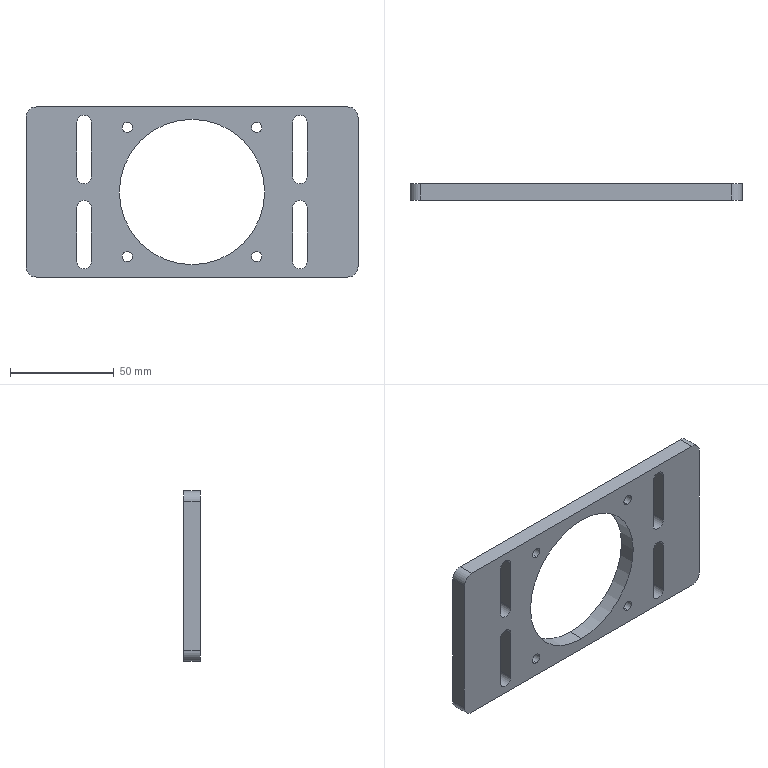Part | SolidWorks | features HoleWzd 2, Extrusion 1, Fillet 1, ICE 1 | 1 solid | 40 faces | box 160 x 8 x 82 mm | volume 66317 mm3 | cylinder 26 | plane 14 | commonest cylinder face diameters 7 x12 5 x8 10 x4 70 x2
STEP:
#1=CARTESIAN_POINT('',(-31.16,0.,-33.66));
#2=VERTEX_POINT('',#1);
#3=CARTESIAN_POINT('',(-31.16,0.,-28.66));
#4=VERTEX_POINT('',#3);
#5=CARTESIAN_POINT('',(-31.16,0.,-31.16));
#6=DIRECTION('',(0.,1.,0.));
#7=DIRECTION('',(0.,0.,1.));
#8=AXIS2_PLACEMENT_3D('',#5,#6,#7);
#9=CIRCLE('',#8,2.5);
#10=EDGE_CURVE('',#2,#4,#9,.T.);
#11=ORIENTED_EDGE('',*,*,#10,.F.);
#12=CARTESIAN_POINT('',(-31.16,8.,-33.66));
#13=VERTEX_POINT('',#12);
#14=CARTESIAN_POINT('',(-31.16,8.,-33.66));
#15=DIRECTION('',(0.,1.,0.));
#16=VECTOR('',#15,1000.);
#17=LINE('',#14,#16);
#18=EDGE_CURVE('',#2,#13,#17,.T.);
#19=ORIENTED_EDGE('',*,*,#18,.T.);
#20=CARTESIAN_POINT('',(-31.16,8.,-28.66));
#21=VERTEX_POINT('',#20);
#22=CARTESIAN_POINT('',(-31.16,8.,-31.16));
#23=DIRECTION('',(0.,1.,0.));
#24=DIRECTION('',(0.,0.,1.));
#25=AXIS2_PLACEMENT_3D('',#22,#23,#24);
#26=CIRCLE('',#25,2.5);
#27=EDGE_CURVE('',#13,#21,#26,.T.);
#28=ORIENTED_EDGE('',*,*,#27,.T.);
#29=CARTESIAN_POINT('',(-31.16,8.,-28.66));
#30=DIRECTION('',(0.,1.,0.));
#31=VECTOR('',#30,1000.);
#32=LINE('',#29,#31);
#33=EDGE_CURVE('',#4,#21,#32,.T.);
#34=ORIENTED_EDGE('',*,*,#33,.F.);
#35=EDGE_LOOP('',(#11,#19,#28,#34));
#36=FACE_OUTER_BOUND('',#35,.T.);
#37=CARTESIAN_POINT('',(-31.16,8.,-31.16));
#38=DIRECTION('',(0.,1.,0.));
#39=DIRECTION('',(0.,0.,1.));
#40=AXIS2_PLACEMENT_3D('',#37,#38,#39);
#41=CYLINDRICAL_SURFACE('',#40,2.5);
#42=ADVANCED_FACE('',(#36),#41,.F.);
#43=CARTESIAN_POINT('',(31.16,0.,-33.66));
#44=VERTEX_POINT('',#43);
#45=CARTESIAN_POINT('',(31.16,0.,-28.66));
#46=VERTEX_POINT('',#45);
#47=CARTESIAN_POINT('',(31.16,0.,-31.16));
#48=DIRECTION('',(0.,1.,0.));
#49=DIRECTION('',(0.,0.,1.));
#50=AXIS2_PLACEMENT_3D('',#47,#48,#49);
#51=CIRCLE('',#50,2.5);
#52=EDGE_CURVE('',#44,#46,#51,.T.);
#53=ORIENTED_EDGE('',*,*,#52,.F.);
#54=CARTESIAN_POINT('',(31.16,8.,-33.66));
#55=VERTEX_POINT('',#54);
#56=CARTESIAN_POINT('',(31.16,8.,-33.66));
#57=DIRECTION('',(0.,1.,0.));
#58=VECTOR('',#57,1000.);
#59=LINE('',#56,#58);
#60=EDGE_CURVE('',#44,#55,#59,.T.);
#61=ORIENTED_EDGE('',*,*,#60,.T.);
#62=CARTESIAN_POINT('',(31.16,8.,-28.66));
#63=VERTEX_POINT('',#62);
#64=CARTESIAN_POINT('',(31.16,8.,-31.16));
#65=DIRECTION('',(0.,1.,0.));
#66=DIRECTION('',(0.,0.,1.));
#67=AXIS2_PLACEMENT_3D('',#64,#65,#66);
#68=CIRCLE('',#67,2.5);
#69=EDGE_CURVE('',#55,#63,#68,.T.);
#70=ORIENTED_EDGE('',*,*,#69,.T.);
#71=CARTESIAN_POINT('',(31.16,8.,-28.66));
#72=DIRECTION('',(0.,1.,0.));
#73=VECTOR('',#72,1000.);
#74=LINE('',#71,#73);
#75=EDGE_CURVE('',#46,#63,#74,.T.);
#76=ORIENTED_EDGE('',*,*,#75,.F.);
#77=EDGE_LOOP('',(#53,#61,#70,#76));
#78=FACE_OUTER_BOUND('',#77,.T.);
#79=CARTESIAN_POINT('',(31.16,8.,-31.16));
#80=DIRECTION('',(0.,1.,0.));
#81=DIRECTION('',(0.,0.,1.));
#82=AXIS2_PLACEMENT_3D('',#79,#80,#81);
#83=CYLINDRICAL_SURFACE('',#82,2.5);
#84=ADVANCED_FACE('',(#78),#83,.F.);
#85=CARTESIAN_POINT('',(31.16,0.,28.66));
#86=VERTEX_POINT('',#85);
#87=CARTESIAN_POINT('',(31.16,0.,33.66));
#88=VERTEX_POINT('',#87);
#89=CARTESIAN_POINT('',(31.16,0.,31.16));
#90=DIRECTION('',(0.,1.,0.));
#91=DIRECTION('',(0.,0.,1.));
#92=AXIS2_PLACEMENT_3D('',#89,#90,#91);
#93=CIRCLE('',#92,2.5);
#94=EDGE_CURVE('',#86,#88,#93,.T.);
#95=ORIENTED_EDGE('',*,*,#94,.F.);
#96=CARTESIAN_POINT('',(31.16,8.,28.66));
#97=VERTEX_POINT('',#96);
#98=CARTESIAN_POINT('',(31.16,8.,28.66));
#99=DIRECTION('',(0.,1.,0.));
#100=VECTOR('',#99,1000.);
#101=LINE('',#98,#100);
#102=EDGE_CURVE('',#86,#97,#101,.T.);
#103=ORIENTED_EDGE('',*,*,#102,.T.);
#104=CARTESIAN_POINT('',(31.16,8.,33.66));
#105=VERTEX_POINT('',#104);
#106=CARTESIAN_POINT('',(31.16,8.,31.16));
#107=DIRECTION('',(0.,1.,0.));
#108=DIRECTION('',(0.,0.,1.));
#109=AXIS2_PLACEMENT_3D('',#106,#107,#108);
#110=CIRCLE('',#109,2.5);
#111=EDGE_CURVE('',#97,#105,#110,.T.);
#112=ORIENTED_EDGE('',*,*,#111,.T.);
#113=CARTESIAN_POINT('',(31.16,8.,33.66));
#114=DIRECTION('',(0.,1.,0.));
#115=VECTOR('',#114,1000.);
#116=LINE('',#113,#115);
#117=EDGE_CURVE('',#88,#105,#116,.T.);
#118=ORIENTED_EDGE('',*,*,#117,.F.);
#119=EDGE_LOOP('',(#95,#103,#112,#118));
#120=FACE_OUTER_BOUND('',#119,.T.);
#121=CARTESIAN_POINT('',(31.16,8.,31.16));
#122=DIRECTION('',(0.,1.,0.));
#123=DIRECTION('',(0.,0.,1.));
#124=AXIS2_PLACEMENT_3D('',#121,#122,#123);
#125=CYLINDRICAL_SURFACE('',#124,2.5);
#126=ADVANCED_FACE('',(#120),#125,.F.);
#127=CARTESIAN_POINT('',(-31.16,0.,28.66));
#128=VERTEX_POINT('',#127);
#129=CARTESIAN_POINT('',(-31.16,0.,33.66));
#130=VERTEX_POINT('',#129);
#131=CARTESIAN_POINT('',(-31.16,0.,31.16));
#132=DIRECTION('',(0.,1.,0.));
#133=DIRECTION('',(0.,0.,1.));
#134=AXIS2_PLACEMENT_3D('',#131,#132,#133);
#135=CIRCLE('',#134,2.5);
#136=EDGE_CURVE('',#128,#130,#135,.T.);
#137=ORIENTED_EDGE('',*,*,#136,.F.);
#138=CARTESIAN_POINT('',(-31.16,8.,28.66));
#139=VERTEX_POINT('',#138);
#140=CARTESIAN_POINT('',(-31.16,8.,28.66));
#141=DIRECTION('',(0.,1.,0.));
#142=VECTOR('',#141,1000.);
#143=LINE('',#140,#142);
#144=EDGE_CURVE('',#128,#139,#143,.T.);
#145=ORIENTED_EDGE('',*,*,#144,.T.);
#146=CARTESIAN_POINT('',(-31.16,8.,33.66));
#147=VERTEX_POINT('',#146);
#148=CARTESIAN_POINT('',(-31.16,8.,31.16));
#149=DIRECTION('',(0.,1.,0.));
#150=DIRECTION('',(0.,0.,1.));
#151=AXIS2_PLACEMENT_3D('',#148,#149,#150);
#152=CIRCLE('',#151,2.5);
#153=EDGE_CURVE('',#139,#147,#152,.T.);
#154=ORIENTED_EDGE('',*,*,#153,.T.);
#155=CARTESIAN_POINT('',(-31.16,8.,33.66));
#156=DIRECTION('',(0.,1.,0.));
#157=VECTOR('',#156,1000.);
#158=LINE('',#155,#157);
#159=EDGE_CURVE('',#130,#147,#158,.T.);
#160=ORIENTED_EDGE('',*,*,#159,.F.);
#161=EDGE_LOOP('',(#137,#145,#154,#160));
#162=FACE_OUTER_BOUND('',#161,.T.);
#163=CARTESIAN_POINT('',(-31.16,8.,31.16));
#164=DIRECTION('',(0.,1.,0.));
#165=DIRECTION('',(0.,0.,1.));
#166=AXIS2_PLACEMENT_3D('',#163,#164,#165);
#167=CYLINDRICAL_SURFACE('',#166,2.5);
#168=ADVANCED_FACE('',(#162),#167,.F.);
#169=CARTESIAN_POINT('',(0.,0.,-35.));
#170=VERTEX_POINT('',#169);
#171=CARTESIAN_POINT('',(0.,0.,35.));
#172=VERTEX_POINT('',#171);
#173=CARTESIAN_POINT('',(0.,0.,0.));
#174=DIRECTION('',(0.,1.,0.));
#175=DIRECTION('',(0.,0.,1.));
#176=AXIS2_PLACEMENT_3D('',#173,#174,#175);
#177=CIRCLE('',#176,35.);
#178=EDGE_CURVE('',#170,#172,#177,.T.);
#179=ORIENTED_EDGE('',*,*,#178,.F.);
#180=CARTESIAN_POINT('',(0.,8.,-35.));
#181=VERTEX_POINT('',#180);
#182=CARTESIAN_POINT('',(0.,0.,-35.));
#183=DIRECTION('',(0.,1.,0.));
#184=VECTOR('',#183,1000.);
#185=LINE('',#182,#184);
#186=EDGE_CURVE('',#170,#181,#185,.T.);
#187=ORIENTED_EDGE('',*,*,#186,.T.);
#188=CARTESIAN_POINT('',(0.,8.,35.));
#189=VERTEX_POINT('',#188);
#190=CARTESIAN_POINT('',(0.,8.,0.));
#191=DIRECTION('',(0.,1.,0.));
#192=DIRECTION('',(0.,0.,1.));
#193=AXIS2_PLACEMENT_3D('',#190,#191,#192);
#194=CIRCLE('',#193,35.);
#195=EDGE_CURVE('',#181,#189,#194,.T.);
#196=ORIENTED_EDGE('',*,*,#195,.T.);
#197=CARTESIAN_POINT('',(0.,0.,35.));
#198=DIRECTION('',(0.,1.,0.));
#199=VECTOR('',#198,1000.);
#200=LINE('',#197,#199);
#201=EDGE_CURVE('',#172,#189,#200,.T.);
#202=ORIENTED_EDGE('',*,*,#201,.F.);
#203=EDGE_LOOP('',(#179,#187,#196,#202));
#204=FACE_OUTER_BOUND('',#203,.T.);
#205=CARTESIAN_POINT('',(0.,0.,0.));
#206=DIRECTION('',(0.,1.,0.));
#207=DIRECTION('',(0.,0.,1.));
#208=AXIS2_PLACEMENT_3D('',#205,#206,#207);
#209=CYLINDRICAL_SURFACE('',#208,35.);
#210=ADVANCED_FACE('',(#204),#209,.F.);
#211=CARTESIAN_POINT('',(-52.,0.,-4.));
#212=VERTEX_POINT('',#211);
#213=CARTESIAN_POINT('',(-48.5,0.,-7.5));
#214=VERTEX_POINT('',#213);
#215=CARTESIAN_POINT('',(-52.,0.,-7.5));
#216=DIRECTION('',(0.,1.,0.));
#217=DIRECTION('',(0.,0.,1.));
#218=AXIS2_PLACEMENT_3D('',#215,#216,#217);
#219=CIRCLE('',#218,3.5);
#220=EDGE_CURVE('',#212,#214,#219,.T.);
#221=ORIENTED_EDGE('',*,*,#220,.F.);
#222=CARTESIAN_POINT('',(-52.,8.,-4.));
#223=VERTEX_POINT('',#222);
#224=CARTESIAN_POINT('',(-52.,8.,-4.));
#225=DIRECTION('',(0.,1.,0.));
#226=VECTOR('',#225,1000.);
#227=LINE('',#224,#226);
#228=EDGE_CURVE('',#212,#223,#227,.T.);
#229=ORIENTED_EDGE('',*,*,#228,.T.);
#230=CARTESIAN_POINT('',(-48.5,8.,-7.5));
#231=VERTEX_POINT('',#230);
#232=CARTESIAN_POINT('',(-52.,8.,-7.5));
#233=DIRECTION('',(0.,1.,0.));
#234=DIRECTION('',(0.,0.,1.));
#235=AXIS2_PLACEMENT_3D('',#232,#233,#234);
#236=CIRCLE('',#235,3.5);
#237=EDGE_CURVE('',#223,#231,#236,.T.);
#238=ORIENTED_EDGE('',*,*,#237,.T.);
#239=CARTESIAN_POINT('',(-48.5,0.,-7.5));
#240=DIRECTION('',(0.,-1.,0.));
#241=VECTOR('',#240,1000.);
#242=LINE('',#239,#241);
#243=EDGE_CURVE('',#231,#214,#242,.T.);
#244=ORIENTED_EDGE('',*,*,#243,.T.);
#245=EDGE_LOOP('',(#221,#229,#238,#244));
#246=FACE_OUTER_BOUND('',#245,.T.);
#247=CARTESIAN_POINT('',(-52.,8.,-7.5));
#248=DIRECTION('',(0.,1.,0.));
#249=DIRECTION('',(0.,0.,1.));
#250=AXIS2_PLACEMENT_3D('',#247,#248,#249);
#251=CYLINDRICAL_SURFACE('',#250,3.5);
#252=ADVANCED_FACE('',(#246),#251,.F.);
#253=CARTESIAN_POINT('',(-52.,0.,37.));
#254=VERTEX_POINT('',#253);
#255=CARTESIAN_POINT('',(-48.5,0.,33.5));
#256=VERTEX_POINT('',#255);
#257=CARTESIAN_POINT('',(-52.,0.,33.5));
#258=DIRECTION('',(0.,1.,0.));
#259=DIRECTION('',(0.,0.,1.));
#260=AXIS2_PLACEMENT_3D('',#257,#258,#259);
#261=CIRCLE('',#260,3.5);
#262=EDGE_CURVE('',#254,#256,#261,.T.);
#263=ORIENTED_EDGE('',*,*,#262,.F.);
#264=CARTESIAN_POINT('',(-52.,8.,37.));
#265=VERTEX_POINT('',#264);
#266=CARTESIAN_POINT('',(-52.,8.,37.));
#267=DIRECTION('',(0.,1.,0.));
#268=VECTOR('',#267,1000.);
#269=LINE('',#266,#268);
#270=EDGE_CURVE('',#254,#265,#269,.T.);
#271=ORIENTED_EDGE('',*,*,#270,.T.);
#272=CARTESIAN_POINT('',(-48.5,8.,33.5));
#273=VERTEX_POINT('',#272);
#274=CARTESIAN_POINT('',(-52.,8.,33.5));
#275=DIRECTION('',(0.,1.,0.));
#276=DIRECTION('',(0.,0.,1.));
#277=AXIS2_PLACEMENT_3D('',#274,#275,#276);
#278=CIRCLE('',#277,3.5);
#279=EDGE_CURVE('',#265,#273,#278,.T.);
#280=ORIENTED_EDGE('',*,*,#279,.T.);
#281=CARTESIAN_POINT('',(-48.5,0.,33.5));
#282=DIRECTION('',(0.,-1.,0.));
#283=VECTOR('',#282,1000.);
#284=LINE('',#281,#283);
#285=EDGE_CURVE('',#273,#256,#284,.T.);
#286=ORIENTED_EDGE('',*,*,#285,.T.);
#287=EDGE_LOOP('',(#263,#271,#280,#286));
#288=FACE_OUTER_BOUND('',#287,.T.);
#289=CARTESIAN_POINT('',(-52.,8.,33.5));
#290=DIRECTION('',(0.,1.,0.));
#291=DIRECTION('',(0.,0.,1.));
#292=AXIS2_PLACEMENT_3D('',#289,#290,#291);
#293=CYLINDRICAL_SURFACE('',#292,3.5);
#294=ADVANCED_FACE('',(#288),#293,.F.);
#295=CARTESIAN_POINT('',(52.,0.,37.));
#296=VERTEX_POINT('',#295);
#297=CARTESIAN_POINT('',(55.5,0.,33.5));
#298=VERTEX_POINT('',#297);
#299=CARTESIAN_POINT('',(52.,0.,33.5));
#300=DIRECTION('',(0.,1.,0.));
#301=DIRECTION('',(0.,0.,1.));
#302=AXIS2_PLACEMENT_3D('',#299,#300,#301);
#303=CIRCLE('',#302,3.5);
#304=EDGE_CURVE('',#296,#298,#303,.T.);
#305=ORIENTED_EDGE('',*,*,#304,.F.);
#306=CARTESIAN_POINT('',(52.,8.,37.));
#307=VERTEX_POINT('',#306);
#308=CARTESIAN_POINT('',(52.,8.,37.));
#309=DIRECTION('',(0.,1.,0.));
#310=VECTOR('',#309,1000.);
#311=LINE('',#308,#310);
#312=EDGE_CURVE('',#296,#307,#311,.T.);
#313=ORIENTED_EDGE('',*,*,#312,.T.);
#314=CARTESIAN_POINT('',(55.5,8.,33.5));
#315=VERTEX_POINT('',#314);
#316=CARTESIAN_POINT('',(52.,8.,33.5));
#317=DIRECTION('',(0.,1.,0.));
#318=DIRECTION('',(0.,0.,1.));
#319=AXIS2_PLACEMENT_3D('',#316,#317,#318);
#320=CIRCLE('',#319,3.5);
#321=EDGE_CURVE('',#307,#315,#320,.T.);
#322=ORIENTED_EDGE('',*,*,#321,.T.);
#323=CARTESIAN_POINT('',(55.5,0.,33.5));
#324=DIRECTION('',(0.,-1.,0.));
#325=VECTOR('',#324,1000.);
#326=LINE('',#323,#325);
#327=EDGE_CURVE('',#315,#298,#326,.T.);
#328=ORIENTED_EDGE('',*,*,#327,.T.);
#329=EDGE_LOOP('',(#305,#313,#322,#328));
#330=FACE_OUTER_BOUND('',#329,.T.);
#331=CARTESIAN_POINT('',(52.,8.,33.5));
#332=DIRECTION('',(0.,1.,0.));
#333=DIRECTION('',(0.,0.,1.));
#334=AXIS2_PLACEMENT_3D('',#331,#332,#333);
#335=CYLINDRICAL_SURFACE('',#334,3.5);
#336=ADVANCED_FACE('',(#330),#335,.F.);
#337=CARTESIAN_POINT('',(52.,0.,-4.));
#338=VERTEX_POINT('',#337);
#339=CARTESIAN_POINT('',(55.5,0.,-7.5));
#340=VERTEX_POINT('',#339);
#341=CARTESIAN_POINT('',(52.,0.,-7.5));
#342=DIRECTION('',(0.,1.,0.));
#343=DIRECTION('',(0.,0.,1.));
#344=AXIS2_PLACEMENT_3D('',#341,#342,#343);
#345=CIRCLE('',#344,3.5);
#346=EDGE_CURVE('',#338,#340,#345,.T.);
#347=ORIENTED_EDGE('',*,*,#346,.F.);
#348=CARTESIAN_POINT('',(52.,8.,-4.));
#349=VERTEX_POINT('',#348);
#350=CARTESIAN_POINT('',(52.,8.,-4.));
#351=DIRECTION('',(0.,1.,0.));
#352=VECTOR('',#351,1000.);
#353=LINE('',#350,#352);
#354=EDGE_CURVE('',#338,#349,#353,.T.);
#355=ORIENTED_EDGE('',*,*,#354,.T.);
#356=CARTESIAN_POINT('',(55.5,8.,-7.5));
#357=VERTEX_POINT('',#356);
#358=CARTESIAN_POINT('',(52.,8.,-7.5));
#359=DIRECTION('',(0.,1.,0.));
#360=DIRECTION('',(0.,0.,1.));
#361=AXIS2_PLACEMENT_3D('',#358,#359,#360);
#362=CIRCLE('',#361,3.5);
#363=EDGE_CURVE('',#349,#357,#362,.T.);
#364=ORIENTED_EDGE('',*,*,#363,.T.);
#365=CARTESIAN_POINT('',(55.5,0.,-7.5));
#366=DIRECTION('',(0.,-1.,0.));
#367=VECTOR('',#366,1000.);
#368=LINE('',#365,#367);
#369=EDGE_CURVE('',#357,#340,#368,.T.);
#370=ORIENTED_EDGE('',*,*,#369,.T.);
#371=EDGE_LOOP('',(#347,#355,#364,#370));
#372=FACE_OUTER_BOUND('',#371,.T.);
#373=CARTESIAN_POINT('',(52.,8.,-7.5));
#374=DIRECTION('',(0.,1.,0.));
#375=DIRECTION('',(0.,0.,1.));
#376=AXIS2_PLACEMENT_3D('',#373,#374,#375);
#377=CYLINDRICAL_SURFACE('',#376,3.5);
#378=ADVANCED_FACE('',(#372),#377,.F.);
#379=CARTESIAN_POINT('',(80.,8.,36.));
#380=VERTEX_POINT('',#379);
#381=CARTESIAN_POINT('',(80.,8.,-36.));
#382=VERTEX_POINT('',#381);
#383=CARTESIAN_POINT('',(80.,8.,41.));
#384=DIRECTION('',(0.,0.,-1.));
#385=VECTOR('',#384,1000.);
#386=LINE('',#383,#385);
#387=EDGE_CURVE('',#380,#382,#386,.T.);
#388=ORIENTED_EDGE('',*,*,#387,.F.);
#389=CARTESIAN_POINT('',(80.,0.,36.));
#390=VERTEX_POINT('',#389);
#391=CARTESIAN_POINT('',(80.,8.,36.));
#392=DIRECTION('',(0.,-1.,0.));
#393=VECTOR('',#392,1000.);
#394=LINE('',#391,#393);
#395=EDGE_CURVE('',#380,#390,#394,.T.);
#396=ORIENTED_EDGE('',*,*,#395,.T.);
#397=CARTESIAN_POINT('',(80.,0.,-36.));
#398=VERTEX_POINT('',#397);
#399=CARTESIAN_POINT('',(80.,0.,41.));
#400=DIRECTION('',(0.,0.,-1.));
#401=VECTOR('',#400,1000.);
#402=LINE('',#399,#401);
#403=EDGE_CURVE('',#390,#398,#402,.T.);
#404=ORIENTED_EDGE('',*,*,#403,.T.);
#405=CARTESIAN_POINT('',(80.,8.,-36.));
#406=DIRECTION('',(0.,1.,0.));
#407=VECTOR('',#406,1000.);
#408=LINE('',#405,#407);
#409=EDGE_CURVE('',#398,#382,#408,.T.);
#410=ORIENTED_EDGE('',*,*,#409,.T.);
#411=EDGE_LOOP('',(#388,#396,#404,#410));
#412=FACE_OUTER_BOUND('',#411,.T.);
#413=CARTESIAN_POINT('',(80.,8.,41.));
#414=DIRECTION('',(-1.,0.,0.));
#415=DIRECTION('',(0.,0.,1.));
#416=AXIS2_PLACEMENT_3D('',#413,#414,#415);
#417=PLANE('',#416);
#418=ADVANCED_FACE('',(#412),#417,.F.);
#419=CARTESIAN_POINT('',(75.,8.,-41.));
#420=VERTEX_POINT('',#419);
#421=CARTESIAN_POINT('',(-75.,8.,-41.));
#422=VERTEX_POINT('',#421);
#423=CARTESIAN_POINT('',(-80.,8.,-41.));
#424=DIRECTION('',(-1.,0.,0.));
#425=VECTOR('',#424,1000.);
#426=LINE('',#423,#425);
#427=EDGE_CURVE('',#420,#422,#426,.T.);
#428=ORIENTED_EDGE('',*,*,#427,.F.);
#429=CARTESIAN_POINT('',(75.,0.,-41.));
#430=VERTEX_POINT('',#429);
#431=CARTESIAN_POINT('',(75.,8.,-41.));
#432=DIRECTION('',(0.,-1.,0.));
#433=VECTOR('',#432,1000.);
#434=LINE('',#431,#433);
#435=EDGE_CURVE('',#420,#430,#434,.T.);
#436=ORIENTED_EDGE('',*,*,#435,.T.);
#437=CARTESIAN_POINT('',(-75.,0.,-41.));
#438=VERTEX_POINT('',#437);
#439=CARTESIAN_POINT('',(-80.,0.,-41.));
#440=DIRECTION('',(-1.,0.,0.));
#441=VECTOR('',#440,1000.);
#442=LINE('',#439,#441);
#443=EDGE_CURVE('',#430,#438,#442,.T.);
#444=ORIENTED_EDGE('',*,*,#443,.T.);
#445=CARTESIAN_POINT('',(-75.,8.,-41.));
#446=DIRECTION('',(0.,1.,0.));
#447=VECTOR('',#446,1000.);
#448=LINE('',#445,#447);
#449=EDGE_CURVE('',#438,#422,#448,.T.);
#450=ORIENTED_EDGE('',*,*,#449,.T.);
#451=EDGE_LOOP('',(#428,#436,#444,#450));
#452=FACE_OUTER_BOUND('',#451,.T.);
#453=CARTESIAN_POINT('',(-80.,8.,-41.));
#454=DIRECTION('',(0.,0.,1.));
#455=DIRECTION('',(1.,0.,0.));
#456=AXIS2_PLACEMENT_3D('',#453,#454,#455);
#457=PLANE('',#456);
#458=ADVANCED_FACE('',(#452),#457,.F.);
#459=CARTESIAN_POINT('',(-80.,0.,-36.));
#460=VERTEX_POINT('',#459);
#461=CARTESIAN_POINT('',(-80.,0.,36.));
#462=VERTEX_POINT('',#461);
#463=CARTESIAN_POINT('',(-80.,0.,41.));
#464=DIRECTION('',(0.,0.,1.));
#465=VECTOR('',#464,1000.);
#466=LINE('',#463,#465);
#467=EDGE_CURVE('',#460,#462,#466,.T.);
#468=ORIENTED_EDGE('',*,*,#467,.T.);
#469=CARTESIAN_POINT('',(-80.,8.,36.));
#470=VERTEX_POINT('',#469);
#471=CARTESIAN_POINT('',(-80.,8.,36.));
#472=DIRECTION('',(0.,1.,0.));
#473=VECTOR('',#472,1000.);
#474=LINE('',#471,#473);
#475=EDGE_CURVE('',#462,#470,#474,.T.);
#476=ORIENTED_EDGE('',*,*,#475,.T.);
#477=CARTESIAN_POINT('',(-80.,8.,-36.));
#478=VERTEX_POINT('',#477);
#479=CARTESIAN_POINT('',(-80.,8.,41.));
#480=DIRECTION('',(0.,0.,1.));
#481=VECTOR('',#480,1000.);
#482=LINE('',#479,#481);
#483=EDGE_CURVE('',#478,#470,#482,.T.);
#484=ORIENTED_EDGE('',*,*,#483,.F.);
#485=CARTESIAN_POINT('',(-80.,8.,-36.));
#486=DIRECTION('',(0.,-1.,0.));
#487=VECTOR('',#486,1000.);
#488=LINE('',#485,#487);
#489=EDGE_CURVE('',#478,#460,#488,.T.);
#490=ORIENTED_EDGE('',*,*,#489,.T.);
#491=EDGE_LOOP('',(#468,#476,#484,#490));
#492=FACE_OUTER_BOUND('',#491,.T.);
#493=CARTESIAN_POINT('',(-80.,8.,41.));
#494=DIRECTION('',(1.,0.,0.));
#495=DIRECTION('',(0.,0.,-1.));
#496=AXIS2_PLACEMENT_3D('',#493,#494,#495);
#497=PLANE('',#496);
#498=ADVANCED_FACE('',(#492),#497,.F.);
#499=CARTESIAN_POINT('',(-75.,0.,41.));
#500=VERTEX_POINT('',#499);
#501=CARTESIAN_POINT('',(75.,0.,41.));
#502=VERTEX_POINT('',#501);
#503=CARTESIAN_POINT('',(-80.,0.,41.));
#504=DIRECTION('',(1.,0.,0.));
#505=VECTOR('',#504,1000.);
#506=LINE('',#503,#505);
#507=EDGE_CURVE('',#500,#502,#506,.T.);
#508=ORIENTED_EDGE('',*,*,#507,.T.);
#509=CARTESIAN_POINT('',(75.,8.,41.));
#510=VERTEX_POINT('',#509);
#511=CARTESIAN_POINT('',(75.,8.,41.));
#512=DIRECTION('',(0.,1.,0.));
#513=VECTOR('',#512,1000.);
#514=LINE('',#511,#513);
#515=EDGE_CURVE('',#502,#510,#514,.T.);
#516=ORIENTED_EDGE('',*,*,#515,.T.);
#517=CARTESIAN_POINT('',(-75.,8.,41.));
#518=VERTEX_POINT('',#517);
#519=CARTESIAN_POINT('',(-80.,8.,41.));
#520=DIRECTION('',(1.,0.,0.));
#521=VECTOR('',#520,1000.);
#522=LINE('',#519,#521);
#523=EDGE_CURVE('',#518,#510,#522,.T.);
#524=ORIENTED_EDGE('',*,*,#523,.F.);
#525=CARTESIAN_POINT('',(-75.,8.,41.));
#526=DIRECTION('',(0.,-1.,0.));
#527=VECTOR('',#526,1000.);
#528=LINE('',#525,#527);
#529=EDGE_CURVE('',#518,#500,#528,.T.);
#530=ORIENTED_EDGE('',*,*,#529,.T.);
#531=EDGE_LOOP('',(#508,#516,#524,#530));
#532=FACE_OUTER_BOUND('',#531,.T.);
#533=CARTESIAN_POINT('',(-80.,8.,41.));
#534=DIRECTION('',(0.,0.,-1.));
#535=DIRECTION('',(-1.,0.,0.));
#536=AXIS2_PLACEMENT_3D('',#533,#534,#535);
#537=PLANE('',#536);
#538=ADVANCED_FACE('',(#532),#537,.F.);
#539=CARTESIAN_POINT('',(-31.16,8.,-31.16));
#540=DIRECTION('',(0.,1.,0.));
#541=DIRECTION('',(0.,0.,1.));
#542=AXIS2_PLACEMENT_3D('',#539,#540,#541);
#543=CIRCLE('',#542,2.5);
#544=EDGE_CURVE('',#21,#13,#543,.T.);
#545=ORIENTED_EDGE('',*,*,#544,.F.);
#546=ORIENTED_EDGE('',*,*,#27,.F.);
#547=EDGE_LOOP('',(#545,#546));
#548=FACE_BOUND('',#547,.T.);
#549=CARTESIAN_POINT('',(31.16,8.,-31.16));
#550=DIRECTION('',(0.,1.,0.));
#551=DIRECTION('',(0.,0.,1.));
#552=AXIS2_PLACEMENT_3D('',#549,#550,#551);
#553=CIRCLE('',#552,2.5);
#554=EDGE_CURVE('',#63,#55,#553,.T.);
#555=ORIENTED_EDGE('',*,*,#554,.F.);
#556=ORIENTED_EDGE('',*,*,#69,.F.);
#557=EDGE_LOOP('',(#555,#556));
#558=FACE_BOUND('',#557,.T.);
#559=CARTESIAN_POINT('',(31.16,8.,31.16));
#560=DIRECTION('',(0.,1.,0.));
#561=DIRECTION('',(0.,0.,1.));
#562=AXIS2_PLACEMENT_3D('',#559,#560,#561);
#563=CIRCLE('',#562,2.5);
#564=EDGE_CURVE('',#105,#97,#563,.T.);
#565=ORIENTED_EDGE('',*,*,#564,.F.);
#566=ORIENTED_EDGE('',*,*,#111,.F.);
#567=EDGE_LOOP('',(#565,#566));
#568=FACE_BOUND('',#567,.T.);
#569=CARTESIAN_POINT('',(-31.16,8.,31.16));
#570=DIRECTION('',(0.,1.,0.));
#571=DIRECTION('',(0.,0.,1.));
#572=AXIS2_PLACEMENT_3D('',#569,#570,#571);
#573=CIRCLE('',#572,2.5);
#574=EDGE_CURVE('',#147,#139,#573,.T.);
#575=ORIENTED_EDGE('',*,*,#574,.F.);
#576=ORIENTED_EDGE('',*,*,#153,.F.);
#577=EDGE_LOOP('',(#575,#576));
#578=FACE_BOUND('',#577,.T.);
#579=CARTESIAN_POINT('',(0.,8.,0.));
#580=DIRECTION('',(0.,1.,0.));
#581=DIRECTION('',(0.,0.,1.));
#582=AXIS2_PLACEMENT_3D('',#579,#580,#581);
#583=CIRCLE('',#582,35.);
#584=EDGE_CURVE('',#189,#181,#583,.T.);
#585=ORIENTED_EDGE('',*,*,#584,.F.);
#586=ORIENTED_EDGE('',*,*,#195,.F.);
#587=EDGE_LOOP('',(#585,#586));
#588=FACE_BOUND('',#587,.T.);
#589=CARTESIAN_POINT('',(-55.5,8.,-7.5));
#590=VERTEX_POINT('',#589);
#591=CARTESIAN_POINT('',(-52.,8.,-7.5));
#592=DIRECTION('',(0.,1.,0.));
#593=DIRECTION('',(0.,0.,1.));
#594=AXIS2_PLACEMENT_3D('',#591,#592,#593);
#595=CIRCLE('',#594,3.5);
#596=EDGE_CURVE('',#590,#223,#595,.T.);
#597=ORIENTED_EDGE('',*,*,#596,.F.);
#598=CARTESIAN_POINT('',(-55.5,8.,-33.5));
#599=VERTEX_POINT('',#598);
#600=CARTESIAN_POINT('',(-55.5,8.,-7.5));
#601=DIRECTION('',(0.,0.,-1.));
#602=VECTOR('',#601,1000.);
#603=LINE('',#600,#602);
#604=EDGE_CURVE('',#590,#599,#603,.T.);
#605=ORIENTED_EDGE('',*,*,#604,.T.);
#606=CARTESIAN_POINT('',(-48.5,8.,-33.5));
#607=VERTEX_POINT('',#606);
#608=CARTESIAN_POINT('',(-52.,8.,-33.5));
#609=DIRECTION('',(0.,1.,0.));
#610=DIRECTION('',(0.,0.,1.));
#611=AXIS2_PLACEMENT_3D('',#608,#609,#610);
#612=CIRCLE('',#611,3.5);
#613=EDGE_CURVE('',#607,#599,#612,.T.);
#614=ORIENTED_EDGE('',*,*,#613,.F.);
#615=CARTESIAN_POINT('',(-48.5,8.,-7.5));
#616=DIRECTION('',(0.,0.,-1.));
#617=VECTOR('',#616,1000.);
#618=LINE('',#615,#617);
#619=EDGE_CURVE('',#231,#607,#618,.T.);
#620=ORIENTED_EDGE('',*,*,#619,.F.);
#621=ORIENTED_EDGE('',*,*,#237,.F.);
#622=EDGE_LOOP('',(#597,#605,#614,#620,#621));
#623=FACE_BOUND('',#622,.T.);
#624=CARTESIAN_POINT('',(-48.5,8.,7.5));
#625=VERTEX_POINT('',#624);
#626=CARTESIAN_POINT('',(-48.5,8.,33.5));
#627=DIRECTION('',(0.,0.,-1.));
#628=VECTOR('',#627,1000.);
#629=LINE('',#626,#628);
#630=EDGE_CURVE('',#273,#625,#629,.T.);
#631=ORIENTED_EDGE('',*,*,#630,.F.);
#632=ORIENTED_EDGE('',*,*,#279,.F.);
#633=CARTESIAN_POINT('',(-55.5,8.,33.5));
#634=VERTEX_POINT('',#633);
#635=CARTESIAN_POINT('',(-52.,8.,33.5));
#636=DIRECTION('',(0.,1.,0.));
#637=DIRECTION('',(0.,0.,1.));
#638=AXIS2_PLACEMENT_3D('',#635,#636,#637);
#639=CIRCLE('',#638,3.5);
#640=EDGE_CURVE('',#634,#265,#639,.T.);
#641=ORIENTED_EDGE('',*,*,#640,.F.);
#642=CARTESIAN_POINT('',(-55.5,8.,7.5));
#643=VERTEX_POINT('',#642);
#644=CARTESIAN_POINT('',(-55.5,8.,33.5));
#645=DIRECTION('',(0.,0.,-1.));
#646=VECTOR('',#645,1000.);
#647=LINE('',#644,#646);
#648=EDGE_CURVE('',#634,#643,#647,.T.);
#649=ORIENTED_EDGE('',*,*,#648,.T.);
#650=CARTESIAN_POINT('',(-52.,8.,7.5));
#651=DIRECTION('',(0.,1.,0.));
#652=DIRECTION('',(0.,0.,1.));
#653=AXIS2_PLACEMENT_3D('',#650,#651,#652);
#654=CIRCLE('',#653,3.5);
#655=EDGE_CURVE('',#625,#643,#654,.T.);
#656=ORIENTED_EDGE('',*,*,#655,.F.);
#657=EDGE_LOOP('',(#631,#632,#641,#649,#656));
#658=FACE_BOUND('',#657,.T.);
#659=CARTESIAN_POINT('',(55.5,8.,7.5));
#660=VERTEX_POINT('',#659);
#661=CARTESIAN_POINT('',(55.5,8.,33.5));
#662=DIRECTION('',(0.,0.,-1.));
#663=VECTOR('',#662,1000.);
#664=LINE('',#661,#663);
#665=EDGE_CURVE('',#315,#660,#664,.T.);
#666=ORIENTED_EDGE('',*,*,#665,.F.);
#667=ORIENTED_EDGE('',*,*,#321,.F.);
#668=CARTESIAN_POINT('',(48.5,8.,33.5));
#669=VERTEX_POINT('',#668);
#670=CARTESIAN_POINT('',(52.,8.,33.5));
#671=DIRECTION('',(0.,1.,0.));
#672=DIRECTION('',(0.,0.,1.));
#673=AXIS2_PLACEMENT_3D('',#670,#671,#672);
#674=CIRCLE('',#673,3.5);
#675=EDGE_CURVE('',#669,#307,#674,.T.);
#676=ORIENTED_EDGE('',*,*,#675,.F.);
#677=CARTESIAN_POINT('',(48.5,8.,7.5));
#678=VERTEX_POINT('',#677);
#679=CARTESIAN_POINT('',(48.5,8.,33.5));
#680=DIRECTION('',(0.,0.,-1.));
#681=VECTOR('',#680,1000.);
#682=LINE('',#679,#681);
#683=EDGE_CURVE('',#669,#678,#682,.T.);
#684=ORIENTED_EDGE('',*,*,#683,.T.);
#685=CARTESIAN_POINT('',(52.,8.,7.5));
#686=DIRECTION('',(0.,1.,0.));
#687=DIRECTION('',(0.,0.,1.));
#688=AXIS2_PLACEMENT_3D('',#685,#686,#687);
#689=CIRCLE('',#688,3.5);
#690=EDGE_CURVE('',#660,#678,#689,.T.);
#691=ORIENTED_EDGE('',*,*,#690,.F.);
#692=EDGE_LOOP('',(#666,#667,#676,#684,#691));
#693=FACE_BOUND('',#692,.T.);
#694=CARTESIAN_POINT('',(55.5,8.,-33.5));
#695=VERTEX_POINT('',#694);
#696=CARTESIAN_POINT('',(55.5,8.,-7.5));
#697=DIRECTION('',(0.,0.,-1.));
#698=VECTOR('',#697,1000.);
#699=LINE('',#696,#698);
#700=EDGE_CURVE('',#357,#695,#699,.T.);
#701=ORIENTED_EDGE('',*,*,#700,.F.);
#702=ORIENTED_EDGE('',*,*,#363,.F.);
#703=CARTESIAN_POINT('',(48.5,8.,-7.5));
#704=VERTEX_POINT('',#703);
#705=CARTESIAN_POINT('',(52.,8.,-7.5));
#706=DIRECTION('',(0.,1.,0.));
#707=DIRECTION('',(0.,0.,1.));
#708=AXIS2_PLACEMENT_3D('',#705,#706,#707);
#709=CIRCLE('',#708,3.5);
#710=EDGE_CURVE('',#704,#349,#709,.T.);
#711=ORIENTED_EDGE('',*,*,#710,.F.);
#712=CARTESIAN_POINT('',(48.5,8.,-33.5));
#713=VERTEX_POINT('',#712);
#714=CARTESIAN_POINT('',(48.5,8.,-7.5));
#715=DIRECTION('',(0.,0.,-1.));
#716=VECTOR('',#715,1000.);
#717=LINE('',#714,#716);
#718=EDGE_CURVE('',#704,#713,#717,.T.);
#719=ORIENTED_EDGE('',*,*,#718,.T.);
#720=CARTESIAN_POINT('',(52.,8.,-33.5));
#721=DIRECTION('',(0.,1.,0.));
#722=DIRECTION('',(0.,0.,1.));
#723=AXIS2_PLACEMENT_3D('',#720,#721,#722);
#724=CIRCLE('',#723,3.5);
#725=EDGE_CURVE('',#695,#713,#724,.T.);
#726=ORIENTED_EDGE('',*,*,#725,.F.);
#727=EDGE_LOOP('',(#701,#702,#711,#719,#726));
#728=FACE_BOUND('',#727,.T.);
#729=ORIENTED_EDGE('',*,*,#523,.T.);
#730=CARTESIAN_POINT('',(75.,8.,36.));
#731=DIRECTION('',(0.,1.,0.));
#732=DIRECTION('',(0.,0.,-1.));
#733=AXIS2_PLACEMENT_3D('',#730,#731,#732);
#734=CIRCLE('',#733,5.);
#735=EDGE_CURVE('',#510,#380,#734,.T.);
#736=ORIENTED_EDGE('',*,*,#735,.T.);
#737=ORIENTED_EDGE('',*,*,#387,.T.);
#738=CARTESIAN_POINT('',(75.,8.,-36.));
#739=DIRECTION('',(0.,1.,0.));
#740=DIRECTION('',(0.,0.,-1.));
#741=AXIS2_PLACEMENT_3D('',#738,#739,#740);
#742=CIRCLE('',#741,5.);
#743=EDGE_CURVE('',#382,#420,#742,.T.);
#744=ORIENTED_EDGE('',*,*,#743,.T.);
#745=ORIENTED_EDGE('',*,*,#427,.T.);
#746=CARTESIAN_POINT('',(-75.,8.,-36.));
#747=DIRECTION('',(0.,1.,0.));
#748=DIRECTION('',(0.,0.,-1.));
#749=AXIS2_PLACEMENT_3D('',#746,#747,#748);
#750=CIRCLE('',#749,5.);
#751=EDGE_CURVE('',#422,#478,#750,.T.);
#752=ORIENTED_EDGE('',*,*,#751,.T.);
#753=ORIENTED_EDGE('',*,*,#483,.T.);
#754=CARTESIAN_POINT('',(-75.,8.,36.));
#755=DIRECTION('',(0.,1.,0.));
#756=DIRECTION('',(0.,0.,-1.));
#757=AXIS2_PLACEMENT_3D('',#754,#755,#756);
#758=CIRCLE('',#757,5.);
#759=EDGE_CURVE('',#470,#518,#758,.T.);
#760=ORIENTED_EDGE('',*,*,#759,.T.);
#761=EDGE_LOOP('',(#729,#736,#737,#744,#745,#752,#753,#760));
#762=FACE_OUTER_BOUND('',#761,.T.);
#763=CARTESIAN_POINT('',(0.,8.,0.));
#764=DIRECTION('',(0.,-1.,0.));
#765=DIRECTION('',(0.,0.,-1.));
#766=AXIS2_PLACEMENT_3D('',#763,#764,#765);
#767=PLANE('',#766);
#768=ADVANCED_FACE('',(#548,#558,#568,#578,#588,#623,#658,#693,#728,#762),#767,.F.);
#769=CARTESIAN_POINT('',(-31.16,0.,-31.16));
#770=DIRECTION('',(0.,1.,0.));
#771=DIRECTION('',(0.,0.,1.));
#772=AXIS2_PLACEMENT_3D('',#769,#770,#771);
#773=CIRCLE('',#772,2.5);
#774=EDGE_CURVE('',#4,#2,#773,.T.);
#775=ORIENTED_EDGE('',*,*,#774,.T.);
#776=ORIENTED_EDGE('',*,*,#10,.T.);
#777=EDGE_LOOP('',(#775,#776));
#778=FACE_BOUND('',#777,.T.);
#779=CARTESIAN_POINT('',(31.16,0.,-31.16));
#780=DIRECTION('',(0.,1.,0.));
#781=DIRECTION('',(0.,0.,1.));
#782=AXIS2_PLACEMENT_3D('',#779,#780,#781);
#783=CIRCLE('',#782,2.5);
#784=EDGE_CURVE('',#46,#44,#783,.T.);
#785=ORIENTED_EDGE('',*,*,#784,.T.);
#786=ORIENTED_EDGE('',*,*,#52,.T.);
#787=EDGE_LOOP('',(#785,#786));
#788=FACE_BOUND('',#787,.T.);
#789=CARTESIAN_POINT('',(31.16,0.,31.16));
#790=DIRECTION('',(0.,1.,0.));
#791=DIRECTION('',(0.,0.,1.));
#792=AXIS2_PLACEMENT_3D('',#789,#790,#791);
#793=CIRCLE('',#792,2.5);
#794=EDGE_CURVE('',#88,#86,#793,.T.);
#795=ORIENTED_EDGE('',*,*,#794,.T.);
#796=ORIENTED_EDGE('',*,*,#94,.T.);
#797=EDGE_LOOP('',(#795,#796));
#798=FACE_BOUND('',#797,.T.);
#799=CARTESIAN_POINT('',(-31.16,0.,31.16));
#800=DIRECTION('',(0.,1.,0.));
#801=DIRECTION('',(0.,0.,1.));
#802=AXIS2_PLACEMENT_3D('',#799,#800,#801);
#803=CIRCLE('',#802,2.5);
#804=EDGE_CURVE('',#130,#128,#803,.T.);
#805=ORIENTED_EDGE('',*,*,#804,.T.);
#806=ORIENTED_EDGE('',*,*,#136,.T.);
#807=EDGE_LOOP('',(#805,#806));
#808=FACE_BOUND('',#807,.T.);
#809=CARTESIAN_POINT('',(0.,0.,0.));
#810=DIRECTION('',(0.,1.,0.));
#811=DIRECTION('',(0.,0.,1.));
#812=AXIS2_PLACEMENT_3D('',#809,#810,#811);
#813=CIRCLE('',#812,35.);
#814=EDGE_CURVE('',#172,#170,#813,.T.);
#815=ORIENTED_EDGE('',*,*,#814,.T.);
#816=ORIENTED_EDGE('',*,*,#178,.T.);
#817=EDGE_LOOP('',(#815,#816));
#818=FACE_BOUND('',#817,.T.);
#819=CARTESIAN_POINT('',(-48.5,0.,-33.5));
#820=VERTEX_POINT('',#819);
#821=CARTESIAN_POINT('',(-55.5,0.,-33.5));
#822=VERTEX_POINT('',#821);
#823=CARTESIAN_POINT('',(-52.,0.,-33.5));
#824=DIRECTION('',(0.,1.,0.));
#825=DIRECTION('',(0.,0.,1.));
#826=AXIS2_PLACEMENT_3D('',#823,#824,#825);
#827=CIRCLE('',#826,3.5);
#828=EDGE_CURVE('',#820,#822,#827,.T.);
#829=ORIENTED_EDGE('',*,*,#828,.T.);
#830=CARTESIAN_POINT('',(-55.5,0.,-7.5));
#831=VERTEX_POINT('',#830);
#832=CARTESIAN_POINT('',(-55.5,0.,-7.5));
#833=DIRECTION('',(0.,0.,-1.));
#834=VECTOR('',#833,1000.);
#835=LINE('',#832,#834);
#836=EDGE_CURVE('',#831,#822,#835,.T.);
#837=ORIENTED_EDGE('',*,*,#836,.F.);
#838=CARTESIAN_POINT('',(-52.,0.,-7.5));
#839=DIRECTION('',(0.,1.,0.));
#840=DIRECTION('',(0.,0.,1.));
#841=AXIS2_PLACEMENT_3D('',#838,#839,#840);
#842=CIRCLE('',#841,3.5);
#843=EDGE_CURVE('',#831,#212,#842,.T.);
#844=ORIENTED_EDGE('',*,*,#843,.T.);
#845=ORIENTED_EDGE('',*,*,#220,.T.);
#846=CARTESIAN_POINT('',(-48.5,0.,-7.5));
#847=DIRECTION('',(0.,0.,-1.));
#848=VECTOR('',#847,1000.);
#849=LINE('',#846,#848);
#850=EDGE_CURVE('',#214,#820,#849,.T.);
#851=ORIENTED_EDGE('',*,*,#850,.T.);
#852=EDGE_LOOP('',(#829,#837,#844,#845,#851));
#853=FACE_BOUND('',#852,.T.);
#854=CARTESIAN_POINT('',(-48.5,0.,7.5));
#855=VERTEX_POINT('',#854);
#856=CARTESIAN_POINT('',(-55.5,0.,7.5));
#857=VERTEX_POINT('',#856);
#858=CARTESIAN_POINT('',(-52.,0.,7.5));
#859=DIRECTION('',(0.,1.,0.));
#860=DIRECTION('',(0.,0.,1.));
#861=AXIS2_PLACEMENT_3D('',#858,#859,#860);
#862=CIRCLE('',#861,3.5);
#863=EDGE_CURVE('',#855,#857,#862,.T.);
#864=ORIENTED_EDGE('',*,*,#863,.T.);
#865=CARTESIAN_POINT('',(-55.5,0.,33.5));
#866=VERTEX_POINT('',#865);
#867=CARTESIAN_POINT('',(-55.5,0.,33.5));
#868=DIRECTION('',(0.,0.,-1.));
#869=VECTOR('',#868,1000.);
#870=LINE('',#867,#869);
#871=EDGE_CURVE('',#866,#857,#870,.T.);
#872=ORIENTED_EDGE('',*,*,#871,.F.);
#873=CARTESIAN_POINT('',(-52.,0.,33.5));
#874=DIRECTION('',(0.,1.,0.));
#875=DIRECTION('',(0.,0.,1.));
#876=AXIS2_PLACEMENT_3D('',#873,#874,#875);
#877=CIRCLE('',#876,3.5);
#878=EDGE_CURVE('',#866,#254,#877,.T.);
#879=ORIENTED_EDGE('',*,*,#878,.T.);
#880=ORIENTED_EDGE('',*,*,#262,.T.);
#881=CARTESIAN_POINT('',(-48.5,0.,33.5));
#882=DIRECTION('',(0.,0.,-1.));
#883=VECTOR('',#882,1000.);
#884=LINE('',#881,#883);
#885=EDGE_CURVE('',#256,#855,#884,.T.);
#886=ORIENTED_EDGE('',*,*,#885,.T.);
#887=EDGE_LOOP('',(#864,#872,#879,#880,#886));
#888=FACE_BOUND('',#887,.T.);
#889=CARTESIAN_POINT('',(48.5,0.,33.5));
#890=VERTEX_POINT('',#889);
#891=CARTESIAN_POINT('',(48.5,0.,7.5));
#892=VERTEX_POINT('',#891);
#893=CARTESIAN_POINT('',(48.5,0.,33.5));
#894=DIRECTION('',(0.,0.,-1.));
#895=VECTOR('',#894,1000.);
#896=LINE('',#893,#895);
#897=EDGE_CURVE('',#890,#892,#896,.T.);
#898=ORIENTED_EDGE('',*,*,#897,.F.);
#899=CARTESIAN_POINT('',(52.,0.,33.5));
#900=DIRECTION('',(0.,1.,0.));
#901=DIRECTION('',(0.,0.,1.));
#902=AXIS2_PLACEMENT_3D('',#899,#900,#901);
#903=CIRCLE('',#902,3.5);
#904=EDGE_CURVE('',#890,#296,#903,.T.);
#905=ORIENTED_EDGE('',*,*,#904,.T.);
#906=ORIENTED_EDGE('',*,*,#304,.T.);
#907=CARTESIAN_POINT('',(55.5,0.,7.5));
#908=VERTEX_POINT('',#907);
#909=CARTESIAN_POINT('',(55.5,0.,33.5));
#910=DIRECTION('',(0.,0.,-1.));
#911=VECTOR('',#910,1000.);
#912=LINE('',#909,#911);
#913=EDGE_CURVE('',#298,#908,#912,.T.);
#914=ORIENTED_EDGE('',*,*,#913,.T.);
#915=CARTESIAN_POINT('',(52.,0.,7.5));
#916=DIRECTION('',(0.,1.,0.));
#917=DIRECTION('',(0.,0.,1.));
#918=AXIS2_PLACEMENT_3D('',#915,#916,#917);
#919=CIRCLE('',#918,3.5);
#920=EDGE_CURVE('',#908,#892,#919,.T.);
#921=ORIENTED_EDGE('',*,*,#920,.T.);
#922=EDGE_LOOP('',(#898,#905,#906,#914,#921));
#923=FACE_BOUND('',#922,.T.);
#924=CARTESIAN_POINT('',(55.5,0.,-33.5));
#925=VERTEX_POINT('',#924);
#926=CARTESIAN_POINT('',(48.5,0.,-33.5));
#927=VERTEX_POINT('',#926);
#928=CARTESIAN_POINT('',(52.,0.,-33.5));
#929=DIRECTION('',(0.,1.,0.));
#930=DIRECTION('',(0.,0.,1.));
#931=AXIS2_PLACEMENT_3D('',#928,#929,#930);
#932=CIRCLE('',#931,3.5);
#933=EDGE_CURVE('',#925,#927,#932,.T.);
#934=ORIENTED_EDGE('',*,*,#933,.T.);
#935=CARTESIAN_POINT('',(48.5,0.,-7.5));
#936=VERTEX_POINT('',#935);
#937=CARTESIAN_POINT('',(48.5,0.,-7.5));
#938=DIRECTION('',(0.,0.,-1.));
#939=VECTOR('',#938,1000.);
#940=LINE('',#937,#939);
#941=EDGE_CURVE('',#936,#927,#940,.T.);
#942=ORIENTED_EDGE('',*,*,#941,.F.);
#943=CARTESIAN_POINT('',(52.,0.,-7.5));
#944=DIRECTION('',(0.,1.,0.));
#945=DIRECTION('',(0.,0.,1.));
#946=AXIS2_PLACEMENT_3D('',#943,#944,#945);
#947=CIRCLE('',#946,3.5);
#948=EDGE_CURVE('',#936,#338,#947,.T.);
#949=ORIENTED_EDGE('',*,*,#948,.T.);
#950=ORIENTED_EDGE('',*,*,#346,.T.);
#951=CARTESIAN_POINT('',(55.5,0.,-7.5));
#952=DIRECTION('',(0.,0.,-1.));
#953=VECTOR('',#952,1000.);
#954=LINE('',#951,#953);
#955=EDGE_CURVE('',#340,#925,#954,.T.);
#956=ORIENTED_EDGE('',*,*,#955,.T.);
#957=EDGE_LOOP('',(#934,#942,#949,#950,#956));
#958=FACE_BOUND('',#957,.T.);
#959=ORIENTED_EDGE('',*,*,#403,.F.);
#960=CARTESIAN_POINT('',(75.,0.,36.));
#961=DIRECTION('',(0.,-1.,0.));
#962=DIRECTION('',(0.,0.,-1.));
#963=AXIS2_PLACEMENT_3D('',#960,#961,#962);
#964=CIRCLE('',#963,5.);
#965=EDGE_CURVE('',#390,#502,#964,.T.);
#966=ORIENTED_EDGE('',*,*,#965,.T.);
#967=ORIENTED_EDGE('',*,*,#507,.F.);
#968=CARTESIAN_POINT('',(-75.,0.,36.));
#969=DIRECTION('',(0.,-1.,0.));
#970=DIRECTION('',(0.,0.,-1.));
#971=AXIS2_PLACEMENT_3D('',#968,#969,#970);
#972=CIRCLE('',#971,5.);
#973=EDGE_CURVE('',#500,#462,#972,.T.);
#974=ORIENTED_EDGE('',*,*,#973,.T.);
#975=ORIENTED_EDGE('',*,*,#467,.F.);
#976=CARTESIAN_POINT('',(-75.,0.,-36.));
#977=DIRECTION('',(0.,-1.,0.));
#978=DIRECTION('',(0.,0.,-1.));
#979=AXIS2_PLACEMENT_3D('',#976,#977,#978);
#980=CIRCLE('',#979,5.);
#981=EDGE_CURVE('',#460,#438,#980,.T.);
#982=ORIENTED_EDGE('',*,*,#981,.T.);
#983=ORIENTED_EDGE('',*,*,#443,.F.);
#984=CARTESIAN_POINT('',(75.,0.,-36.));
#985=DIRECTION('',(0.,-1.,0.));
#986=DIRECTION('',(0.,0.,-1.));
#987=AXIS2_PLACEMENT_3D('',#984,#985,#986);
#988=CIRCLE('',#987,5.);
#989=EDGE_CURVE('',#430,#398,#988,.T.);
#990=ORIENTED_EDGE('',*,*,#989,.T.);
#991=EDGE_LOOP('',(#959,#966,#967,#974,#975,#982,#983,#990));
#992=FACE_OUTER_BOUND('',#991,.T.);
#993=CARTESIAN_POINT('',(0.,0.,0.));
#994=DIRECTION('',(0.,-1.,0.));
#995=DIRECTION('',(0.,0.,-1.));
#996=AXIS2_PLACEMENT_3D('',#993,#994,#995);
#997=PLANE('',#996);
#998=ADVANCED_FACE('',(#778,#788,#798,#808,#818,#853,#888,#923,#958,#992),#997,.T.);
#999=ORIENTED_EDGE('',*,*,#933,.F.);
#1000=CARTESIAN_POINT('',(55.5,0.,-33.5));
#1001=DIRECTION('',(0.,-1.,0.));
#1002=VECTOR('',#1001,1000.);
#1003=LINE('',#1000,#1002);
#1004=EDGE_CURVE('',#695,#925,#1003,.T.);
#1005=ORIENTED_EDGE('',*,*,#1004,.F.);
#1006=ORIENTED_EDGE('',*,*,#725,.T.);
#1007=CARTESIAN_POINT('',(48.5,8.,-33.5));
#1008=DIRECTION('',(0.,1.,0.));
#1009=VECTOR('',#1008,1000.);
#1010=LINE('',#1007,#1009);
#1011=EDGE_CURVE('',#927,#713,#1010,.T.);
#1012=ORIENTED_EDGE('',*,*,#1011,.F.);
#1013=EDGE_LOOP('',(#999,#1005,#1006,#1012));
#1014=FACE_OUTER_BOUND('',#1013,.T.);
#1015=CARTESIAN_POINT('',(52.,8.,-33.5));
#1016=DIRECTION('',(0.,1.,0.));
#1017=DIRECTION('',(0.,0.,1.));
#1018=AXIS2_PLACEMENT_3D('',#1015,#1016,#1017);
#1019=CYLINDRICAL_SURFACE('',#1018,3.5);
#1020=ADVANCED_FACE('',(#1014),#1019,.F.);
#1021=ORIENTED_EDGE('',*,*,#354,.F.);
#1022=ORIENTED_EDGE('',*,*,#948,.F.);
#1023=CARTESIAN_POINT('',(48.5,8.,-7.5));
#1024=DIRECTION('',(0.,-1.,0.));
#1025=VECTOR('',#1024,1000.);
#1026=LINE('',#1023,#1025);
#1027=EDGE_CURVE('',#704,#936,#1026,.T.);
#1028=ORIENTED_EDGE('',*,*,#1027,.F.);
#1029=ORIENTED_EDGE('',*,*,#710,.T.);
#1030=EDGE_LOOP('',(#1021,#1022,#1028,#1029));
#1031=FACE_OUTER_BOUND('',#1030,.T.);
#1032=CARTESIAN_POINT('',(52.,8.,-7.5));
#1033=DIRECTION('',(0.,1.,0.));
#1034=DIRECTION('',(0.,0.,1.));
#1035=AXIS2_PLACEMENT_3D('',#1032,#1033,#1034);
#1036=CYLINDRICAL_SURFACE('',#1035,3.5);
#1037=ADVANCED_FACE('',(#1031),#1036,.F.);
#1038=ORIENTED_EDGE('',*,*,#1011,.T.);
#1039=ORIENTED_EDGE('',*,*,#718,.F.);
#1040=ORIENTED_EDGE('',*,*,#1027,.T.);
#1041=ORIENTED_EDGE('',*,*,#941,.T.);
#1042=EDGE_LOOP('',(#1038,#1039,#1040,#1041));
#1043=FACE_OUTER_BOUND('',#1042,.T.);
#1044=CARTESIAN_POINT('',(48.5,8.,-7.5));
#1045=DIRECTION('',(-1.,0.,0.));
#1046=DIRECTION('',(0.,0.,1.));
#1047=AXIS2_PLACEMENT_3D('',#1044,#1045,#1046);
#1048=PLANE('',#1047);
#1049=ADVANCED_FACE('',(#1043),#1048,.F.);
#1050=ORIENTED_EDGE('',*,*,#1004,.T.);
#1051=ORIENTED_EDGE('',*,*,#955,.F.);
#1052=ORIENTED_EDGE('',*,*,#369,.F.);
#1053=ORIENTED_EDGE('',*,*,#700,.T.);
#1054=EDGE_LOOP('',(#1050,#1051,#1052,#1053));
#1055=FACE_OUTER_BOUND('',#1054,.T.);
#1056=CARTESIAN_POINT('',(55.5,0.,-7.5));
#1057=DIRECTION('',(1.,0.,0.));
#1058=DIRECTION('',(0.,0.,-1.));
#1059=AXIS2_PLACEMENT_3D('',#1056,#1057,#1058);
#1060=PLANE('',#1059);
#1061=ADVANCED_FACE('',(#1055),#1060,.F.);
#1062=ORIENTED_EDGE('',*,*,#920,.F.);
#1063=CARTESIAN_POINT('',(55.5,0.,7.5));
#1064=DIRECTION('',(0.,-1.,0.));
#1065=VECTOR('',#1064,1000.);
#1066=LINE('',#1063,#1065);
#1067=EDGE_CURVE('',#660,#908,#1066,.T.);
#1068=ORIENTED_EDGE('',*,*,#1067,.F.);
#1069=ORIENTED_EDGE('',*,*,#690,.T.);
#1070=CARTESIAN_POINT('',(48.5,8.,7.5));
#1071=DIRECTION('',(0.,1.,0.));
#1072=VECTOR('',#1071,1000.);
#1073=LINE('',#1070,#1072);
#1074=EDGE_CURVE('',#892,#678,#1073,.T.);
#1075=ORIENTED_EDGE('',*,*,#1074,.F.);
#1076=EDGE_LOOP('',(#1062,#1068,#1069,#1075));
#1077=FACE_OUTER_BOUND('',#1076,.T.);
#1078=CARTESIAN_POINT('',(52.,8.,7.5));
#1079=DIRECTION('',(0.,1.,0.));
#1080=DIRECTION('',(0.,0.,1.));
#1081=AXIS2_PLACEMENT_3D('',#1078,#1079,#1080);
#1082=CYLINDRICAL_SURFACE('',#1081,3.5);
#1083=ADVANCED_FACE('',(#1077),#1082,.F.);
#1084=ORIENTED_EDGE('',*,*,#312,.F.);
#1085=ORIENTED_EDGE('',*,*,#904,.F.);
#1086=CARTESIAN_POINT('',(48.5,8.,33.5));
#1087=DIRECTION('',(0.,-1.,0.));
#1088=VECTOR('',#1087,1000.);
#1089=LINE('',#1086,#1088);
#1090=EDGE_CURVE('',#669,#890,#1089,.T.);
#1091=ORIENTED_EDGE('',*,*,#1090,.F.);
#1092=ORIENTED_EDGE('',*,*,#675,.T.);
#1093=EDGE_LOOP('',(#1084,#1085,#1091,#1092));
#1094=FACE_OUTER_BOUND('',#1093,.T.);
#1095=CARTESIAN_POINT('',(52.,8.,33.5));
#1096=DIRECTION('',(0.,1.,0.));
#1097=DIRECTION('',(0.,0.,1.));
#1098=AXIS2_PLACEMENT_3D('',#1095,#1096,#1097);
#1099=CYLINDRICAL_SURFACE('',#1098,3.5);
#1100=ADVANCED_FACE('',(#1094),#1099,.F.);
#1101=ORIENTED_EDGE('',*,*,#1074,.T.);
#1102=ORIENTED_EDGE('',*,*,#683,.F.);
#1103=ORIENTED_EDGE('',*,*,#1090,.T.);
#1104=ORIENTED_EDGE('',*,*,#897,.T.);
#1105=EDGE_LOOP('',(#1101,#1102,#1103,#1104));
#1106=FACE_OUTER_BOUND('',#1105,.T.);
#1107=CARTESIAN_POINT('',(48.5,8.,33.5));
#1108=DIRECTION('',(-1.,0.,0.));
#1109=DIRECTION('',(0.,0.,1.));
#1110=AXIS2_PLACEMENT_3D('',#1107,#1108,#1109);
#1111=PLANE('',#1110);
#1112=ADVANCED_FACE('',(#1106),#1111,.F.);
#1113=ORIENTED_EDGE('',*,*,#1067,.T.);
#1114=ORIENTED_EDGE('',*,*,#913,.F.);
#1115=ORIENTED_EDGE('',*,*,#327,.F.);
#1116=ORIENTED_EDGE('',*,*,#665,.T.);
#1117=EDGE_LOOP('',(#1113,#1114,#1115,#1116));
#1118=FACE_OUTER_BOUND('',#1117,.T.);
#1119=CARTESIAN_POINT('',(55.5,0.,33.5));
#1120=DIRECTION('',(1.,0.,0.));
#1121=DIRECTION('',(0.,1.,0.));
#1122=AXIS2_PLACEMENT_3D('',#1119,#1120,#1121);
#1123=PLANE('',#1122);
#1124=ADVANCED_FACE('',(#1118),#1123,.F.);
#1125=ORIENTED_EDGE('',*,*,#863,.F.);
#1126=CARTESIAN_POINT('',(-48.5,0.,7.5));
#1127=DIRECTION('',(0.,-1.,0.));
#1128=VECTOR('',#1127,1000.);
#1129=LINE('',#1126,#1128);
#1130=EDGE_CURVE('',#625,#855,#1129,.T.);
#1131=ORIENTED_EDGE('',*,*,#1130,.F.);
#1132=ORIENTED_EDGE('',*,*,#655,.T.);
#1133=CARTESIAN_POINT('',(-55.5,8.,7.5));
#1134=DIRECTION('',(0.,1.,0.));
#1135=VECTOR('',#1134,1000.);
#1136=LINE('',#1133,#1135);
#1137=EDGE_CURVE('',#857,#643,#1136,.T.);
#1138=ORIENTED_EDGE('',*,*,#1137,.F.);
#1139=EDGE_LOOP('',(#1125,#1131,#1132,#1138));
#1140=FACE_OUTER_BOUND('',#1139,.T.);
#1141=CARTESIAN_POINT('',(-52.,8.,7.5));
#1142=DIRECTION('',(0.,1.,0.));
#1143=DIRECTION('',(0.,0.,1.));
#1144=AXIS2_PLACEMENT_3D('',#1141,#1142,#1143);
#1145=CYLINDRICAL_SURFACE('',#1144,3.5);
#1146=ADVANCED_FACE('',(#1140),#1145,.F.);
#1147=ORIENTED_EDGE('',*,*,#270,.F.);
#1148=ORIENTED_EDGE('',*,*,#878,.F.);
#1149=CARTESIAN_POINT('',(-55.5,8.,33.5));
#1150=DIRECTION('',(0.,-1.,0.));
#1151=VECTOR('',#1150,1000.);
#1152=LINE('',#1149,#1151);
#1153=EDGE_CURVE('',#634,#866,#1152,.T.);
#1154=ORIENTED_EDGE('',*,*,#1153,.F.);
#1155=ORIENTED_EDGE('',*,*,#640,.T.);
#1156=EDGE_LOOP('',(#1147,#1148,#1154,#1155));
#1157=FACE_OUTER_BOUND('',#1156,.T.);
#1158=CARTESIAN_POINT('',(-52.,8.,33.5));
#1159=DIRECTION('',(0.,1.,0.));
#1160=DIRECTION('',(0.,0.,1.));
#1161=AXIS2_PLACEMENT_3D('',#1158,#1159,#1160);
#1162=CYLINDRICAL_SURFACE('',#1161,3.5);
#1163=ADVANCED_FACE('',(#1157),#1162,.F.);
#1164=ORIENTED_EDGE('',*,*,#1137,.T.);
#1165=ORIENTED_EDGE('',*,*,#648,.F.);
#1166=ORIENTED_EDGE('',*,*,#1153,.T.);
#1167=ORIENTED_EDGE('',*,*,#871,.T.);
#1168=EDGE_LOOP('',(#1164,#1165,#1166,#1167));
#1169=FACE_OUTER_BOUND('',#1168,.T.);
#1170=CARTESIAN_POINT('',(-55.5,8.,33.5));
#1171=DIRECTION('',(-1.,0.,0.));
#1172=DIRECTION('',(0.,0.,1.));
#1173=AXIS2_PLACEMENT_3D('',#1170,#1171,#1172);
#1174=PLANE('',#1173);
#1175=ADVANCED_FACE('',(#1169),#1174,.F.);
#1176=ORIENTED_EDGE('',*,*,#1130,.T.);
#1177=ORIENTED_EDGE('',*,*,#885,.F.);
#1178=ORIENTED_EDGE('',*,*,#285,.F.);
#1179=ORIENTED_EDGE('',*,*,#630,.T.);
#1180=EDGE_LOOP('',(#1176,#1177,#1178,#1179));
#1181=FACE_OUTER_BOUND('',#1180,.T.);
#1182=CARTESIAN_POINT('',(-48.5,0.,33.5));
#1183=DIRECTION('',(1.,0.,0.));
#1184=DIRECTION('',(0.,1.,0.));
#1185=AXIS2_PLACEMENT_3D('',#1182,#1183,#1184);
#1186=PLANE('',#1185);
#1187=ADVANCED_FACE('',(#1181),#1186,.F.);
#1188=ORIENTED_EDGE('',*,*,#828,.F.);
#1189=CARTESIAN_POINT('',(-48.5,0.,-33.5));
#1190=DIRECTION('',(0.,-1.,0.));
#1191=VECTOR('',#1190,1000.);
#1192=LINE('',#1189,#1191);
#1193=EDGE_CURVE('',#607,#820,#1192,.T.);
#1194=ORIENTED_EDGE('',*,*,#1193,.F.);
#1195=ORIENTED_EDGE('',*,*,#613,.T.);
#1196=CARTESIAN_POINT('',(-55.5,8.,-33.5));
#1197=DIRECTION('',(0.,1.,0.));
#1198=VECTOR('',#1197,1000.);
#1199=LINE('',#1196,#1198);
#1200=EDGE_CURVE('',#822,#599,#1199,.T.);
#1201=ORIENTED_EDGE('',*,*,#1200,.F.);
#1202=EDGE_LOOP('',(#1188,#1194,#1195,#1201));
#1203=FACE_OUTER_BOUND('',#1202,.T.);
#1204=CARTESIAN_POINT('',(-52.,8.,-33.5));
#1205=DIRECTION('',(0.,1.,0.));
#1206=DIRECTION('',(0.,0.,1.));
#1207=AXIS2_PLACEMENT_3D('',#1204,#1205,#1206);
#1208=CYLINDRICAL_SURFACE('',#1207,3.5);
#1209=ADVANCED_FACE('',(#1203),#1208,.F.);
#1210=ORIENTED_EDGE('',*,*,#228,.F.);
#1211=ORIENTED_EDGE('',*,*,#843,.F.);
#1212=CARTESIAN_POINT('',(-55.5,8.,-7.5));
#1213=DIRECTION('',(0.,-1.,0.));
#1214=VECTOR('',#1213,1000.);
#1215=LINE('',#1212,#1214);
#1216=EDGE_CURVE('',#590,#831,#1215,.T.);
#1217=ORIENTED_EDGE('',*,*,#1216,.F.);
#1218=ORIENTED_EDGE('',*,*,#596,.T.);
#1219=EDGE_LOOP('',(#1210,#1211,#1217,#1218));
#1220=FACE_OUTER_BOUND('',#1219,.T.);
#1221=CARTESIAN_POINT('',(-52.,8.,-7.5));
#1222=DIRECTION('',(0.,1.,0.));
#1223=DIRECTION('',(0.,0.,1.));
#1224=AXIS2_PLACEMENT_3D('',#1221,#1222,#1223);
#1225=CYLINDRICAL_SURFACE('',#1224,3.5);
#1226=ADVANCED_FACE('',(#1220),#1225,.F.);
#1227=ORIENTED_EDGE('',*,*,#1200,.T.);
#1228=ORIENTED_EDGE('',*,*,#604,.F.);
#1229=ORIENTED_EDGE('',*,*,#1216,.T.);
#1230=ORIENTED_EDGE('',*,*,#836,.T.);
#1231=EDGE_LOOP('',(#1227,#1228,#1229,#1230));
#1232=FACE_OUTER_BOUND('',#1231,.T.);
#1233=CARTESIAN_POINT('',(-55.5,8.,-7.5));
#1234=DIRECTION('',(-1.,0.,0.));
#1235=DIRECTION('',(0.,0.,1.));
#1236=AXIS2_PLACEMENT_3D('',#1233,#1234,#1235);
#1237=PLANE('',#1236);
#1238=ADVANCED_FACE('',(#1232),#1237,.F.);
#1239=ORIENTED_EDGE('',*,*,#1193,.T.);
#1240=ORIENTED_EDGE('',*,*,#850,.F.);
#1241=ORIENTED_EDGE('',*,*,#243,.F.);
#1242=ORIENTED_EDGE('',*,*,#619,.T.);
#1243=EDGE_LOOP('',(#1239,#1240,#1241,#1242));
#1244=FACE_OUTER_BOUND('',#1243,.T.);
#1245=CARTESIAN_POINT('',(-48.5,0.,-7.5));
#1246=DIRECTION('',(1.,0.,0.));
#1247=DIRECTION('',(0.,0.,-1.));
#1248=AXIS2_PLACEMENT_3D('',#1245,#1246,#1247);
#1249=PLANE('',#1248);
#1250=ADVANCED_FACE('',(#1244),#1249,.F.);
#1251=ORIENTED_EDGE('',*,*,#735,.F.);
#1252=ORIENTED_EDGE('',*,*,#515,.F.);
#1253=ORIENTED_EDGE('',*,*,#965,.F.);
#1254=ORIENTED_EDGE('',*,*,#395,.F.);
#1255=EDGE_LOOP('',(#1251,#1252,#1253,#1254));
#1256=FACE_OUTER_BOUND('',#1255,.T.);
#1257=CARTESIAN_POINT('',(75.,8.,36.));
#1258=DIRECTION('',(0.,-1.,0.));
#1259=DIRECTION('',(0.,0.,-1.));
#1260=AXIS2_PLACEMENT_3D('',#1257,#1258,#1259);
#1261=CYLINDRICAL_SURFACE('',#1260,5.);
#1262=ADVANCED_FACE('',(#1256),#1261,.T.);
#1263=ORIENTED_EDGE('',*,*,#759,.F.);
#1264=ORIENTED_EDGE('',*,*,#475,.F.);
#1265=ORIENTED_EDGE('',*,*,#973,.F.);
#1266=ORIENTED_EDGE('',*,*,#529,.F.);
#1267=EDGE_LOOP('',(#1263,#1264,#1265,#1266));
#1268=FACE_OUTER_BOUND('',#1267,.T.);
#1269=CARTESIAN_POINT('',(-75.,8.,36.));
#1270=DIRECTION('',(0.,-1.,0.));
#1271=DIRECTION('',(0.,0.,-1.));
#1272=AXIS2_PLACEMENT_3D('',#1269,#1270,#1271);
#1273=CYLINDRICAL_SURFACE('',#1272,5.);
#1274=ADVANCED_FACE('',(#1268),#1273,.T.);
#1275=ORIENTED_EDGE('',*,*,#743,.F.);
#1276=ORIENTED_EDGE('',*,*,#409,.F.);
#1277=ORIENTED_EDGE('',*,*,#989,.F.);
#1278=ORIENTED_EDGE('',*,*,#435,.F.);
#1279=EDGE_LOOP('',(#1275,#1276,#1277,#1278));
#1280=FACE_OUTER_BOUND('',#1279,.T.);
#1281=CARTESIAN_POINT('',(75.,8.,-36.));
#1282=DIRECTION('',(0.,-1.,0.));
#1283=DIRECTION('',(0.,0.,-1.));
#1284=AXIS2_PLACEMENT_3D('',#1281,#1282,#1283);
#1285=CYLINDRICAL_SURFACE('',#1284,5.);
#1286=ADVANCED_FACE('',(#1280),#1285,.T.);
#1287=ORIENTED_EDGE('',*,*,#751,.F.);
#1288=ORIENTED_EDGE('',*,*,#449,.F.);
#1289=ORIENTED_EDGE('',*,*,#981,.F.);
#1290=ORIENTED_EDGE('',*,*,#489,.F.);
#1291=EDGE_LOOP('',(#1287,#1288,#1289,#1290));
#1292=FACE_OUTER_BOUND('',#1291,.T.);
#1293=CARTESIAN_POINT('',(-75.,8.,-36.));
#1294=DIRECTION('',(0.,-1.,0.));
#1295=DIRECTION('',(0.,0.,-1.));
#1296=AXIS2_PLACEMENT_3D('',#1293,#1294,#1295);
#1297=CYLINDRICAL_SURFACE('',#1296,5.);
#1298=ADVANCED_FACE('',(#1292),#1297,.T.);
#1299=ORIENTED_EDGE('',*,*,#186,.F.);
#1300=ORIENTED_EDGE('',*,*,#814,.F.);
#1301=ORIENTED_EDGE('',*,*,#201,.T.);
#1302=ORIENTED_EDGE('',*,*,#584,.T.);
#1303=EDGE_LOOP('',(#1299,#1300,#1301,#1302));
#1304=FACE_OUTER_BOUND('',#1303,.T.);
#1305=CARTESIAN_POINT('',(0.,0.,0.));
#1306=DIRECTION('',(0.,1.,0.));
#1307=DIRECTION('',(0.,0.,1.));
#1308=AXIS2_PLACEMENT_3D('',#1305,#1306,#1307);
#1309=CYLINDRICAL_SURFACE('',#1308,35.);
#1310=ADVANCED_FACE('',(#1304),#1309,.F.);
#1311=ORIENTED_EDGE('',*,*,#144,.F.);
#1312=ORIENTED_EDGE('',*,*,#804,.F.);
#1313=ORIENTED_EDGE('',*,*,#159,.T.);
#1314=ORIENTED_EDGE('',*,*,#574,.T.);
#1315=EDGE_LOOP('',(#1311,#1312,#1313,#1314));
#1316=FACE_OUTER_BOUND('',#1315,.T.);
#1317=CARTESIAN_POINT('',(-31.16,8.,31.16));
#1318=DIRECTION('',(0.,1.,0.));
#1319=DIRECTION('',(0.,0.,1.));
#1320=AXIS2_PLACEMENT_3D('',#1317,#1318,#1319);
#1321=CYLINDRICAL_SURFACE('',#1320,2.5);
#1322=ADVANCED_FACE('',(#1316),#1321,.F.);
#1323=ORIENTED_EDGE('',*,*,#102,.F.);
#1324=ORIENTED_EDGE('',*,*,#794,.F.);
#1325=ORIENTED_EDGE('',*,*,#117,.T.);
#1326=ORIENTED_EDGE('',*,*,#564,.T.);
#1327=EDGE_LOOP('',(#1323,#1324,#1325,#1326));
#1328=FACE_OUTER_BOUND('',#1327,.T.);
#1329=CARTESIAN_POINT('',(31.16,8.,31.16));
#1330=DIRECTION('',(0.,1.,0.));
#1331=DIRECTION('',(0.,0.,1.));
#1332=AXIS2_PLACEMENT_3D('',#1329,#1330,#1331);
#1333=CYLINDRICAL_SURFACE('',#1332,2.5);
#1334=ADVANCED_FACE('',(#1328),#1333,.F.);
#1335=ORIENTED_EDGE('',*,*,#60,.F.);
#1336=ORIENTED_EDGE('',*,*,#784,.F.);
#1337=ORIENTED_EDGE('',*,*,#75,.T.);
#1338=ORIENTED_EDGE('',*,*,#554,.T.);
#1339=EDGE_LOOP('',(#1335,#1336,#1337,#1338));
#1340=FACE_OUTER_BOUND('',#1339,.T.);
#1341=CARTESIAN_POINT('',(31.16,8.,-31.16));
#1342=DIRECTION('',(0.,1.,0.));
#1343=DIRECTION('',(0.,0.,1.));
#1344=AXIS2_PLACEMENT_3D('',#1341,#1342,#1343);
#1345=CYLINDRICAL_SURFACE('',#1344,2.5);
#1346=ADVANCED_FACE('',(#1340),#1345,.F.);
#1347=ORIENTED_EDGE('',*,*,#18,.F.);
#1348=ORIENTED_EDGE('',*,*,#774,.F.);
#1349=ORIENTED_EDGE('',*,*,#33,.T.);
#1350=ORIENTED_EDGE('',*,*,#544,.T.);
#1351=EDGE_LOOP('',(#1347,#1348,#1349,#1350));
#1352=FACE_OUTER_BOUND('',#1351,.T.);
#1353=CARTESIAN_POINT('',(-31.16,8.,-31.16));
#1354=DIRECTION('',(0.,1.,0.));
#1355=DIRECTION('',(0.,0.,1.));
#1356=AXIS2_PLACEMENT_3D('',#1353,#1354,#1355);
#1357=CYLINDRICAL_SURFACE('',#1356,2.5);
#1358=ADVANCED_FACE('',(#1352),#1357,.F.);
#1359=CLOSED_SHELL('',(#42,#84,#126,#168,#210,#252,#294,#336,#378,#418,#458,#498,#538,#768,#998,#1020,#1037,#1049,#1061,#1083,#1100,#1112,#1124,#1146,#1163,#1175,#1187,#1209,#1226,#1238,#1250,#1262,#1274,#1286,#1298,#1310,#1322,#1334,#1346,#1358));
#1360=MANIFOLD_SOLID_BREP('',#1359);
#1361=CARTESIAN_POINT('',(0.,0.,0.));
#1362=DIRECTION('',(0.,0.,1.));
#1363=DIRECTION('',(1.,0.,0.));
#1364=AXIS2_PLACEMENT_3D('',#1361,#1362,#1363);
#1365=(LENGTH_UNIT()NAMED_UNIT(*)SI_UNIT(.MILLI.,.METRE.));
#1366=UNCERTAINTY_MEASURE_WITH_UNIT(LENGTH_MEASURE(0.00001),#1365,'','');
#1367=(NAMED_UNIT(*)PLANE_ANGLE_UNIT()SI_UNIT($,.RADIAN.));
#1368=(NAMED_UNIT(*)SI_UNIT($,.STERADIAN.)SOLID_ANGLE_UNIT());
#1369=(GEOMETRIC_REPRESENTATION_CONTEXT(3)GLOBAL_UNCERTAINTY_ASSIGNED_CONTEXT((#1366))GLOBAL_UNIT_ASSIGNED_CONTEXT((#1365,#1367,#1368))REPRESENTATION_CONTEXT('',''));
#1370=ADVANCED_BREP_SHAPE_REPRESENTATION('',(#1360,#1364),#1369);